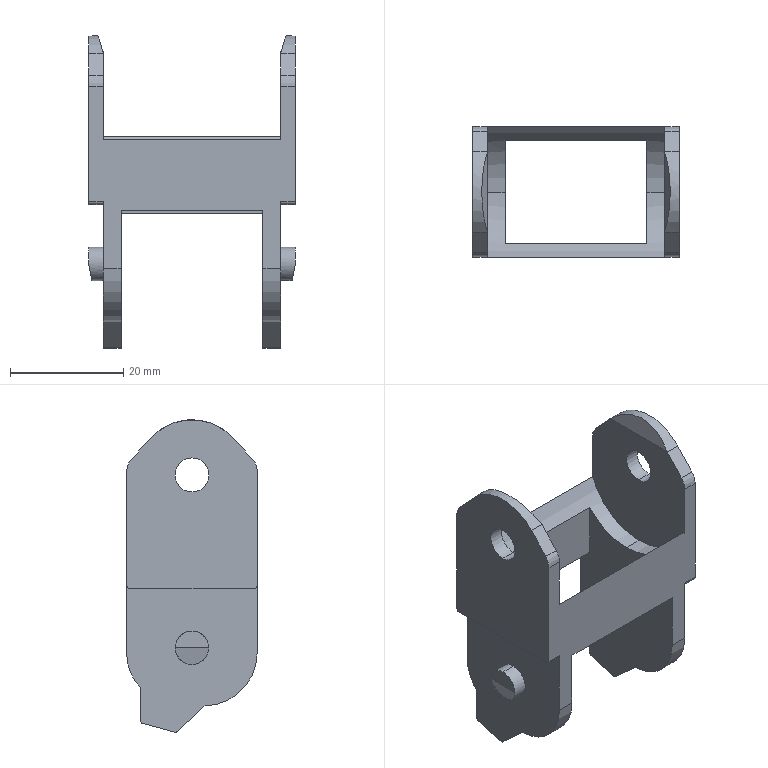Part | SolidWorks | features BaseBody 1 | 1 solid | 62 faces | box 36.5 x 23 x 55.16 mm | volume 8454 mm3 | plane 32 | cylinder 30 | commonest cylinder face diameters 1 x10 6 x8 5.9 x4 16.02 x2 18.716 x2 19.5 x2